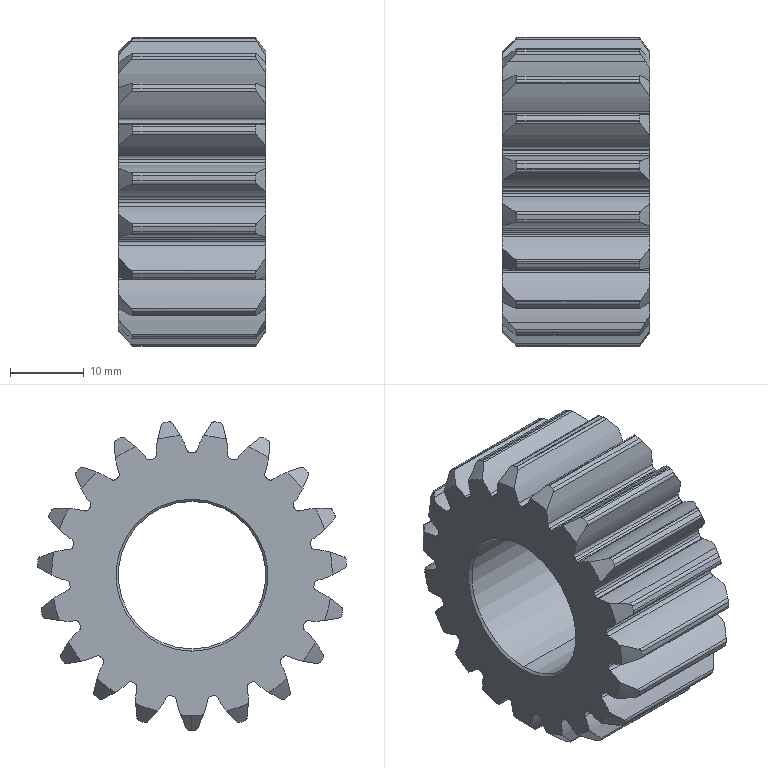Part | SolidWorks | features MBimport 1 | 1 solid | 217 faces | box 20 x 41.909 x 41.772 mm | volume 16148 mm3 | cylinder 171 | cone 44 | plane 2 | commonest cylinder face diameters 1 x90 26.38 x40 33.2 x20 42 x19 20 x2